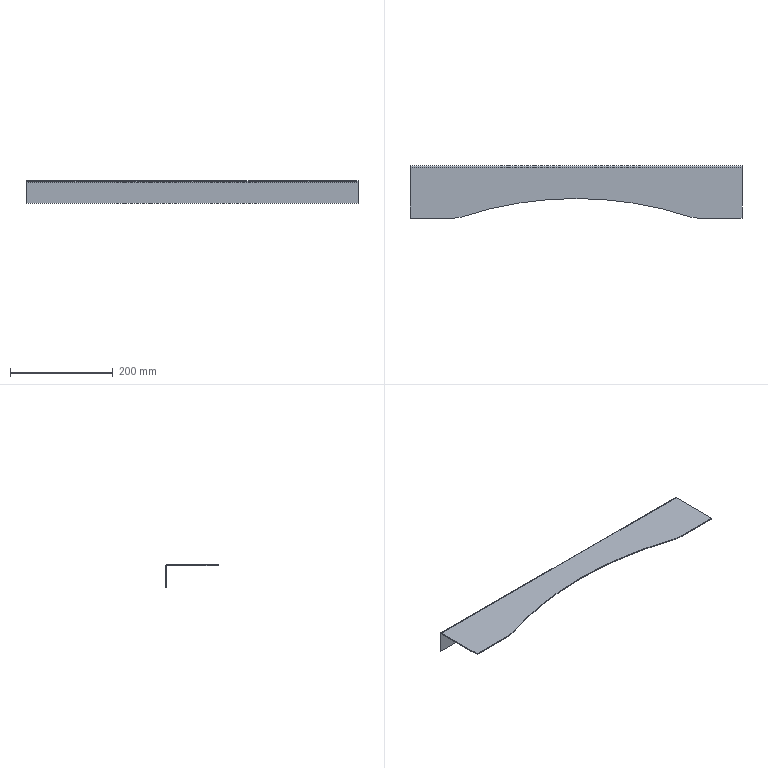Part | NX | features BREP 1 | 1 solid | 18 faces | box 646.176 x 101.6 x 44.45 mm | volume 151816 mm3 | plane 13 | cylinder 5 | commonest cylinder face diameters 127 x2 3.175 x1 6.934 x1 1410 x1
STEP:
#1=CARTESIAN_POINT('',(-238.949,0.,0.));
#2=VERTEX_POINT('',#1);
#3=CARTESIAN_POINT('',(-219.201,3.149,0.));
#4=VERTEX_POINT('',#3);
#5=CARTESIAN_POINT('',(-238.949,63.5,0.));
#6=DIRECTION('',(0.,0.,1.));
#7=DIRECTION('',(0.,-1.,0.));
#8=AXIS2_PLACEMENT_3D('',#5,#6,#7);
#9=CIRCLE('',#8,63.5);
#10=EDGE_CURVE('',#2,#4,#9,.T.);
#11=ORIENTED_EDGE('',*,*,#10,.T.);
#12=CARTESIAN_POINT('',(219.201,3.149,0.));
#13=VERTEX_POINT('',#12);
#14=CARTESIAN_POINT('',(0.,-666.75,0.));
#15=DIRECTION('',(0.,0.,1.));
#16=DIRECTION('',(0.311,0.9504,0.));
#17=AXIS2_PLACEMENT_3D('',#14,#15,#16);
#18=CIRCLE('',#17,704.85);
#19=EDGE_CURVE('',#13,#4,#18,.T.);
#20=ORIENTED_EDGE('',*,*,#19,.F.);
#21=CARTESIAN_POINT('',(238.949,0.,0.));
#22=VERTEX_POINT('',#21);
#23=CARTESIAN_POINT('',(238.949,63.5,0.));
#24=DIRECTION('',(0.,0.,1.));
#25=DIRECTION('',(-0.311,-0.9504,0.));
#26=AXIS2_PLACEMENT_3D('',#23,#24,#25);
#27=CIRCLE('',#26,63.5);
#28=EDGE_CURVE('',#13,#22,#27,.T.);
#29=ORIENTED_EDGE('',*,*,#28,.T.);
#30=CARTESIAN_POINT('',(323.088,0.,0.));
#31=VERTEX_POINT('',#30);
#32=CARTESIAN_POINT('',(238.949,0.,0.));
#33=DIRECTION('',(1.,0.,0.));
#34=VECTOR('',#33,1000.);
#35=LINE('',#32,#34);
#36=EDGE_CURVE('',#22,#31,#35,.T.);
#37=ORIENTED_EDGE('',*,*,#36,.T.);
#38=CARTESIAN_POINT('',(323.088,98.133,0.));
#39=VERTEX_POINT('',#38);
#40=CARTESIAN_POINT('',(323.088,0.,0.));
#41=DIRECTION('',(0.,1.,0.));
#42=VECTOR('',#41,1000.);
#43=LINE('',#40,#42);
#44=EDGE_CURVE('',#31,#39,#43,.T.);
#45=ORIENTED_EDGE('',*,*,#44,.T.);
#46=CARTESIAN_POINT('',(-323.088,98.133,0.));
#47=VERTEX_POINT('',#46);
#48=CARTESIAN_POINT('',(-323.088,98.133,0.));
#49=DIRECTION('',(1.,0.,0.));
#50=VECTOR('',#49,1000.);
#51=LINE('',#48,#50);
#52=EDGE_CURVE('',#47,#39,#51,.T.);
#53=ORIENTED_EDGE('',*,*,#52,.F.);
#54=CARTESIAN_POINT('',(-323.088,0.,0.));
#55=VERTEX_POINT('',#54);
#56=CARTESIAN_POINT('',(-323.088,98.133,0.));
#57=DIRECTION('',(0.,-1.,0.));
#58=VECTOR('',#57,1000.);
#59=LINE('',#56,#58);
#60=EDGE_CURVE('',#47,#55,#59,.T.);
#61=ORIENTED_EDGE('',*,*,#60,.T.);
#62=CARTESIAN_POINT('',(-323.088,0.,0.));
#63=DIRECTION('',(1.,0.,0.));
#64=VECTOR('',#63,1000.);
#65=LINE('',#62,#64);
#66=EDGE_CURVE('',#55,#2,#65,.T.);
#67=ORIENTED_EDGE('',*,*,#66,.T.);
#68=EDGE_LOOP('',(#11,#20,#29,#37,#45,#53,#61,#67));
#69=FACE_BOUND('',#68,.T.);
#70=CARTESIAN_POINT('',(0.,0.,0.));
#71=DIRECTION('',(0.,0.,1.));
#72=DIRECTION('',(1.,0.,0.));
#73=AXIS2_PLACEMENT_3D('',#70,#71,#72);
#74=PLANE('',#73);
#75=ADVANCED_FACE('',(#69),#74,.T.);
#76=CARTESIAN_POINT('',(-323.088,0.,-1.88));
#77=VERTEX_POINT('',#76);
#78=CARTESIAN_POINT('',(-323.088,0.,0.));
#79=DIRECTION('',(0.,0.,-1.));
#80=VECTOR('',#79,1000.);
#81=LINE('',#78,#80);
#82=EDGE_CURVE('',#55,#77,#81,.T.);
#83=ORIENTED_EDGE('',*,*,#82,.T.);
#84=CARTESIAN_POINT('',(-238.949,0.,-1.88));
#85=VERTEX_POINT('',#84);
#86=CARTESIAN_POINT('',(-323.088,0.,-1.88));
#87=DIRECTION('',(1.,0.,0.));
#88=VECTOR('',#87,1000.);
#89=LINE('',#86,#88);
#90=EDGE_CURVE('',#77,#85,#89,.T.);
#91=ORIENTED_EDGE('',*,*,#90,.T.);
#92=CARTESIAN_POINT('',(-238.949,0.,-1.88));
#93=DIRECTION('',(0.,0.,1.));
#94=VECTOR('',#93,1000.);
#95=LINE('',#92,#94);
#96=EDGE_CURVE('',#85,#2,#95,.T.);
#97=ORIENTED_EDGE('',*,*,#96,.T.);
#98=ORIENTED_EDGE('',*,*,#66,.F.);
#99=EDGE_LOOP('',(#83,#91,#97,#98));
#100=FACE_BOUND('',#99,.T.);
#101=CARTESIAN_POINT('',(0.,0.,-0.9398));
#102=DIRECTION('',(0.,-1.,0.));
#103=DIRECTION('',(0.,0.,-1.));
#104=AXIS2_PLACEMENT_3D('',#101,#102,#103);
#105=PLANE('',#104);
#106=ADVANCED_FACE('',(#100),#105,.T.);
#107=CARTESIAN_POINT('',(238.949,0.,-1.88));
#108=VERTEX_POINT('',#107);
#109=CARTESIAN_POINT('',(238.949,0.,-1.88));
#110=DIRECTION('',(0.,0.,1.));
#111=VECTOR('',#110,1000.);
#112=LINE('',#109,#111);
#113=EDGE_CURVE('',#108,#22,#112,.T.);
#114=ORIENTED_EDGE('',*,*,#113,.F.);
#115=CARTESIAN_POINT('',(323.088,0.,-1.88));
#116=VERTEX_POINT('',#115);
#117=CARTESIAN_POINT('',(238.949,0.,-1.88));
#118=DIRECTION('',(1.,0.,0.));
#119=VECTOR('',#118,1000.);
#120=LINE('',#117,#119);
#121=EDGE_CURVE('',#108,#116,#120,.T.);
#122=ORIENTED_EDGE('',*,*,#121,.T.);
#123=CARTESIAN_POINT('',(323.088,0.,0.));
#124=DIRECTION('',(0.,0.,-1.));
#125=VECTOR('',#124,1000.);
#126=LINE('',#123,#125);
#127=EDGE_CURVE('',#31,#116,#126,.T.);
#128=ORIENTED_EDGE('',*,*,#127,.F.);
#129=ORIENTED_EDGE('',*,*,#36,.F.);
#130=EDGE_LOOP('',(#114,#122,#128,#129));
#131=FACE_BOUND('',#130,.T.);
#132=CARTESIAN_POINT('',(0.,0.,-0.9398));
#133=DIRECTION('',(0.,-1.,0.));
#134=DIRECTION('',(0.,0.,-1.));
#135=AXIS2_PLACEMENT_3D('',#132,#133,#134);
#136=PLANE('',#135);
#137=ADVANCED_FACE('',(#131),#136,.T.);
#138=CARTESIAN_POINT('',(-219.201,3.149,-1.88));
#139=VERTEX_POINT('',#138);
#140=CARTESIAN_POINT('',(-238.949,63.5,-1.88));
#141=DIRECTION('',(0.,0.,-1.));
#142=DIRECTION('',(0.311,-0.9504,0.));
#143=AXIS2_PLACEMENT_3D('',#140,#141,#142);
#144=CIRCLE('',#143,63.5);
#145=EDGE_CURVE('',#139,#85,#144,.T.);
#146=ORIENTED_EDGE('',*,*,#145,.F.);
#147=CARTESIAN_POINT('',(-219.201,3.149,-1.88));
#148=DIRECTION('',(0.,0.,1.));
#149=VECTOR('',#148,1000.);
#150=LINE('',#147,#149);
#151=EDGE_CURVE('',#139,#4,#150,.T.);
#152=ORIENTED_EDGE('',*,*,#151,.T.);
#153=ORIENTED_EDGE('',*,*,#10,.F.);
#154=ORIENTED_EDGE('',*,*,#96,.F.);
#155=EDGE_LOOP('',(#146,#152,#153,#154));
#156=FACE_BOUND('',#155,.T.);
#157=CARTESIAN_POINT('',(-238.949,63.5,-2.756));
#158=DIRECTION('',(0.,0.,1.));
#159=DIRECTION('',(0.,-1.,0.));
#160=AXIS2_PLACEMENT_3D('',#157,#158,#159);
#161=CYLINDRICAL_SURFACE('',#160,63.5);
#162=ADVANCED_FACE('',(#156),#161,.T.);
#163=CARTESIAN_POINT('',(219.201,3.149,-1.88));
#164=VERTEX_POINT('',#163);
#165=CARTESIAN_POINT('',(0.,-666.75,-1.88));
#166=DIRECTION('',(0.,0.,1.));
#167=DIRECTION('',(0.311,0.9504,0.));
#168=AXIS2_PLACEMENT_3D('',#165,#166,#167);
#169=CIRCLE('',#168,704.85);
#170=EDGE_CURVE('',#164,#139,#169,.T.);
#171=ORIENTED_EDGE('',*,*,#170,.F.);
#172=CARTESIAN_POINT('',(219.201,3.149,-1.88));
#173=DIRECTION('',(0.,0.,1.));
#174=VECTOR('',#173,1000.);
#175=LINE('',#172,#174);
#176=EDGE_CURVE('',#164,#13,#175,.T.);
#177=ORIENTED_EDGE('',*,*,#176,.T.);
#178=ORIENTED_EDGE('',*,*,#19,.T.);
#179=ORIENTED_EDGE('',*,*,#151,.F.);
#180=EDGE_LOOP('',(#171,#177,#178,#179));
#181=FACE_BOUND('',#180,.T.);
#182=CARTESIAN_POINT('',(0.,-666.75,-0.9398));
#183=DIRECTION('',(0.,0.,1.));
#184=DIRECTION('',(0.3243,0.9459,0.));
#185=AXIS2_PLACEMENT_3D('',#182,#183,#184);
#186=CYLINDRICAL_SURFACE('',#185,704.85);
#187=ADVANCED_FACE('',(#181),#186,.F.);
#188=CARTESIAN_POINT('',(238.949,63.5,-1.88));
#189=DIRECTION('',(0.,0.,-1.));
#190=DIRECTION('',(0.,-1.,0.));
#191=AXIS2_PLACEMENT_3D('',#188,#189,#190);
#192=CIRCLE('',#191,63.5);
#193=EDGE_CURVE('',#108,#164,#192,.T.);
#194=ORIENTED_EDGE('',*,*,#193,.F.);
#195=ORIENTED_EDGE('',*,*,#113,.T.);
#196=ORIENTED_EDGE('',*,*,#28,.F.);
#197=ORIENTED_EDGE('',*,*,#176,.F.);
#198=EDGE_LOOP('',(#194,#195,#196,#197));
#199=FACE_BOUND('',#198,.T.);
#200=CARTESIAN_POINT('',(238.949,63.5,-2.756));
#201=DIRECTION('',(0.,0.,1.));
#202=DIRECTION('',(-0.311,-0.9504,0.));
#203=AXIS2_PLACEMENT_3D('',#200,#201,#202);
#204=CYLINDRICAL_SURFACE('',#203,63.5);
#205=ADVANCED_FACE('',(#199),#204,.T.);
#206=CARTESIAN_POINT('',(-323.088,98.133,-1.88));
#207=VERTEX_POINT('',#206);
#208=CARTESIAN_POINT('',(-323.088,98.133,-1.88));
#209=DIRECTION('',(0.,-1.,0.));
#210=VECTOR('',#209,1000.);
#211=LINE('',#208,#210);
#212=EDGE_CURVE('',#207,#77,#211,.T.);
#213=ORIENTED_EDGE('',*,*,#212,.F.);
#214=CARTESIAN_POINT('',(323.088,98.133,-1.88));
#215=VERTEX_POINT('',#214);
#216=CARTESIAN_POINT('',(-323.088,98.133,-1.88));
#217=DIRECTION('',(1.,0.,0.));
#218=VECTOR('',#217,1000.);
#219=LINE('',#216,#218);
#220=EDGE_CURVE('',#207,#215,#219,.T.);
#221=ORIENTED_EDGE('',*,*,#220,.T.);
#222=CARTESIAN_POINT('',(323.088,0.,-1.88));
#223=DIRECTION('',(0.,1.,0.));
#224=VECTOR('',#223,1000.);
#225=LINE('',#222,#224);
#226=EDGE_CURVE('',#116,#215,#225,.T.);
#227=ORIENTED_EDGE('',*,*,#226,.F.);
#228=ORIENTED_EDGE('',*,*,#121,.F.);
#229=ORIENTED_EDGE('',*,*,#193,.T.);
#230=ORIENTED_EDGE('',*,*,#170,.T.);
#231=ORIENTED_EDGE('',*,*,#145,.T.);
#232=ORIENTED_EDGE('',*,*,#90,.F.);
#233=EDGE_LOOP('',(#213,#221,#227,#228,#229,#230,#231,#232));
#234=FACE_BOUND('',#233,.T.);
#235=CARTESIAN_POINT('',(0.,0.,-1.88));
#236=DIRECTION('',(0.,0.,1.));
#237=DIRECTION('',(1.,0.,0.));
#238=AXIS2_PLACEMENT_3D('',#235,#236,#237);
#239=PLANE('',#238);
#240=ADVANCED_FACE('',(#234),#239,.F.);
#241=ORIENTED_EDGE('',*,*,#127,.T.);
#242=ORIENTED_EDGE('',*,*,#226,.T.);
#243=CARTESIAN_POINT('',(323.088,98.133,0.));
#244=DIRECTION('',(0.,0.,-1.));
#245=VECTOR('',#244,1000.);
#246=LINE('',#243,#245);
#247=EDGE_CURVE('',#39,#215,#246,.T.);
#248=ORIENTED_EDGE('',*,*,#247,.F.);
#249=ORIENTED_EDGE('',*,*,#44,.F.);
#250=EDGE_LOOP('',(#241,#242,#248,#249));
#251=FACE_BOUND('',#250,.T.);
#252=CARTESIAN_POINT('',(323.088,50.8,-0.9398));
#253=DIRECTION('',(1.,0.,0.));
#254=DIRECTION('',(0.,1.,0.));
#255=AXIS2_PLACEMENT_3D('',#252,#253,#254);
#256=PLANE('',#255);
#257=ADVANCED_FACE('',(#251),#256,.T.);
#258=ORIENTED_EDGE('',*,*,#247,.T.);
#259=CARTESIAN_POINT('',(323.088,99.72,-3.467));
#260=VERTEX_POINT('',#259);
#261=CARTESIAN_POINT('',(323.088,98.133,-3.467));
#262=DIRECTION('',(1.,0.,0.));
#263=DIRECTION('',(0.,1.,0.));
#264=AXIS2_PLACEMENT_3D('',#261,#262,#263);
#265=CIRCLE('',#264,1.588);
#266=EDGE_CURVE('',#260,#215,#265,.T.);
#267=ORIENTED_EDGE('',*,*,#266,.F.);
#268=CARTESIAN_POINT('',(323.088,101.6,-3.467));
#269=VERTEX_POINT('',#268);
#270=CARTESIAN_POINT('',(323.088,101.6,-3.467));
#271=DIRECTION('',(0.,-1.,0.));
#272=VECTOR('',#271,1000.);
#273=LINE('',#270,#272);
#274=EDGE_CURVE('',#269,#260,#273,.T.);
#275=ORIENTED_EDGE('',*,*,#274,.F.);
#276=CARTESIAN_POINT('',(323.088,98.133,-3.467));
#277=DIRECTION('',(1.,0.,0.));
#278=DIRECTION('',(0.,1.,0.));
#279=AXIS2_PLACEMENT_3D('',#276,#277,#278);
#280=CIRCLE('',#279,3.467);
#281=EDGE_CURVE('',#269,#39,#280,.T.);
#282=ORIENTED_EDGE('',*,*,#281,.T.);
#283=EDGE_LOOP('',(#258,#267,#275,#282));
#284=FACE_BOUND('',#283,.T.);
#285=CARTESIAN_POINT('',(323.088,99.92,-1.68));
#286=DIRECTION('',(-1.,0.,0.));
#287=DIRECTION('',(0.,0.,1.));
#288=AXIS2_PLACEMENT_3D('',#285,#286,#287);
#289=PLANE('',#288);
#290=ADVANCED_FACE('',(#284),#289,.F.);
#291=CARTESIAN_POINT('',(-323.088,101.6,-3.467));
#292=VERTEX_POINT('',#291);
#293=CARTESIAN_POINT('',(-323.088,98.133,-3.467));
#294=DIRECTION('',(1.,0.,0.));
#295=DIRECTION('',(0.,1.,0.));
#296=AXIS2_PLACEMENT_3D('',#293,#294,#295);
#297=CIRCLE('',#296,3.467);
#298=EDGE_CURVE('',#292,#47,#297,.T.);
#299=ORIENTED_EDGE('',*,*,#298,.T.);
#300=ORIENTED_EDGE('',*,*,#52,.T.);
#301=ORIENTED_EDGE('',*,*,#281,.F.);
#302=CARTESIAN_POINT('',(-323.088,101.6,-3.467));
#303=DIRECTION('',(1.,0.,0.));
#304=VECTOR('',#303,1000.);
#305=LINE('',#302,#304);
#306=EDGE_CURVE('',#292,#269,#305,.T.);
#307=ORIENTED_EDGE('',*,*,#306,.F.);
#308=EDGE_LOOP('',(#299,#300,#301,#307));
#309=FACE_BOUND('',#308,.T.);
#310=CARTESIAN_POINT('',(-323.088,98.133,-3.467));
#311=DIRECTION('',(1.,0.,0.));
#312=DIRECTION('',(0.,1.,0.));
#313=AXIS2_PLACEMENT_3D('',#310,#311,#312);
#314=CYLINDRICAL_SURFACE('',#313,3.467);
#315=ADVANCED_FACE('',(#309),#314,.T.);
#316=CARTESIAN_POINT('',(323.088,101.6,-44.45));
#317=VERTEX_POINT('',#316);
#318=CARTESIAN_POINT('',(-323.088,101.6,-44.45));
#319=VERTEX_POINT('',#318);
#320=CARTESIAN_POINT('',(323.088,101.6,-44.45));
#321=DIRECTION('',(-1.,0.,0.));
#322=VECTOR('',#321,1000.);
#323=LINE('',#320,#322);
#324=EDGE_CURVE('',#317,#319,#323,.T.);
#325=ORIENTED_EDGE('',*,*,#324,.T.);
#326=CARTESIAN_POINT('',(-323.088,101.6,-44.45));
#327=DIRECTION('',(0.,0.,1.));
#328=VECTOR('',#327,1000.);
#329=LINE('',#326,#328);
#330=EDGE_CURVE('',#319,#292,#329,.T.);
#331=ORIENTED_EDGE('',*,*,#330,.T.);
#332=ORIENTED_EDGE('',*,*,#306,.T.);
#333=CARTESIAN_POINT('',(323.088,101.6,-3.467));
#334=DIRECTION('',(0.,0.,-1.));
#335=VECTOR('',#334,1000.);
#336=LINE('',#333,#335);
#337=EDGE_CURVE('',#269,#317,#336,.T.);
#338=ORIENTED_EDGE('',*,*,#337,.T.);
#339=EDGE_LOOP('',(#325,#331,#332,#338));
#340=FACE_BOUND('',#339,.T.);
#341=CARTESIAN_POINT('',(169.557,101.6,0.));
#342=DIRECTION('',(0.,1.,0.));
#343=DIRECTION('',(1.,0.,0.));
#344=AXIS2_PLACEMENT_3D('',#341,#342,#343);
#345=PLANE('',#344);
#346=ADVANCED_FACE('',(#340),#345,.T.);
#347=ORIENTED_EDGE('',*,*,#274,.T.);
#348=CARTESIAN_POINT('',(323.088,99.72,-44.45));
#349=VERTEX_POINT('',#348);
#350=CARTESIAN_POINT('',(323.088,99.72,-3.467));
#351=DIRECTION('',(0.,0.,-1.));
#352=VECTOR('',#351,1000.);
#353=LINE('',#350,#352);
#354=EDGE_CURVE('',#260,#349,#353,.T.);
#355=ORIENTED_EDGE('',*,*,#354,.T.);
#356=CARTESIAN_POINT('',(323.088,101.6,-44.45));
#357=DIRECTION('',(0.,-1.,0.));
#358=VECTOR('',#357,1000.);
#359=LINE('',#356,#358);
#360=EDGE_CURVE('',#317,#349,#359,.T.);
#361=ORIENTED_EDGE('',*,*,#360,.F.);
#362=ORIENTED_EDGE('',*,*,#337,.F.);
#363=EDGE_LOOP('',(#347,#355,#361,#362));
#364=FACE_BOUND('',#363,.T.);
#365=CARTESIAN_POINT('',(323.088,100.66,-23.959));
#366=DIRECTION('',(1.,0.,0.));
#367=DIRECTION('',(0.,1.,0.));
#368=AXIS2_PLACEMENT_3D('',#365,#366,#367);
#369=PLANE('',#368);
#370=ADVANCED_FACE('',(#364),#369,.T.);
#371=ORIENTED_EDGE('',*,*,#360,.T.);
#372=CARTESIAN_POINT('',(-323.088,99.72,-44.45));
#373=VERTEX_POINT('',#372);
#374=CARTESIAN_POINT('',(323.088,99.72,-44.45));
#375=DIRECTION('',(-1.,0.,0.));
#376=VECTOR('',#375,1000.);
#377=LINE('',#374,#376);
#378=EDGE_CURVE('',#349,#373,#377,.T.);
#379=ORIENTED_EDGE('',*,*,#378,.T.);
#380=CARTESIAN_POINT('',(-323.088,101.6,-44.45));
#381=DIRECTION('',(0.,-1.,0.));
#382=VECTOR('',#381,1000.);
#383=LINE('',#380,#382);
#384=EDGE_CURVE('',#319,#373,#383,.T.);
#385=ORIENTED_EDGE('',*,*,#384,.F.);
#386=ORIENTED_EDGE('',*,*,#324,.F.);
#387=EDGE_LOOP('',(#371,#379,#385,#386));
#388=FACE_BOUND('',#387,.T.);
#389=CARTESIAN_POINT('',(0.,100.66,-44.45));
#390=DIRECTION('',(0.,0.,-1.));
#391=DIRECTION('',(0.,-1.,0.));
#392=AXIS2_PLACEMENT_3D('',#389,#390,#391);
#393=PLANE('',#392);
#394=ADVANCED_FACE('',(#388),#393,.T.);
#395=ORIENTED_EDGE('',*,*,#384,.T.);
#396=CARTESIAN_POINT('',(-323.088,99.72,-3.467));
#397=VERTEX_POINT('',#396);
#398=CARTESIAN_POINT('',(-323.088,99.72,-44.45));
#399=DIRECTION('',(0.,0.,1.));
#400=VECTOR('',#399,1000.);
#401=LINE('',#398,#400);
#402=EDGE_CURVE('',#373,#397,#401,.T.);
#403=ORIENTED_EDGE('',*,*,#402,.T.);
#404=CARTESIAN_POINT('',(-323.088,101.6,-3.467));
#405=DIRECTION('',(0.,-1.,0.));
#406=VECTOR('',#405,1000.);
#407=LINE('',#404,#406);
#408=EDGE_CURVE('',#292,#397,#407,.T.);
#409=ORIENTED_EDGE('',*,*,#408,.F.);
#410=ORIENTED_EDGE('',*,*,#330,.F.);
#411=EDGE_LOOP('',(#395,#403,#409,#410));
#412=FACE_BOUND('',#411,.T.);
#413=CARTESIAN_POINT('',(-323.088,100.66,-23.959));
#414=DIRECTION('',(-1.,0.,0.));
#415=DIRECTION('',(0.,0.,1.));
#416=AXIS2_PLACEMENT_3D('',#413,#414,#415);
#417=PLANE('',#416);
#418=ADVANCED_FACE('',(#412),#417,.T.);
#419=ORIENTED_EDGE('',*,*,#408,.T.);
#420=CARTESIAN_POINT('',(-323.088,98.133,-3.467));
#421=DIRECTION('',(1.,0.,0.));
#422=DIRECTION('',(0.,1.,0.));
#423=AXIS2_PLACEMENT_3D('',#420,#421,#422);
#424=CIRCLE('',#423,1.588);
#425=EDGE_CURVE('',#397,#207,#424,.T.);
#426=ORIENTED_EDGE('',*,*,#425,.T.);
#427=CARTESIAN_POINT('',(-323.088,98.133,0.));
#428=DIRECTION('',(0.,0.,-1.));
#429=VECTOR('',#428,1000.);
#430=LINE('',#427,#429);
#431=EDGE_CURVE('',#47,#207,#430,.T.);
#432=ORIENTED_EDGE('',*,*,#431,.F.);
#433=ORIENTED_EDGE('',*,*,#298,.F.);
#434=EDGE_LOOP('',(#419,#426,#432,#433));
#435=FACE_BOUND('',#434,.T.);
#436=CARTESIAN_POINT('',(-323.088,99.92,-1.68));
#437=DIRECTION('',(-1.,0.,0.));
#438=DIRECTION('',(0.,0.,1.));
#439=AXIS2_PLACEMENT_3D('',#436,#437,#438);
#440=PLANE('',#439);
#441=ADVANCED_FACE('',(#435),#440,.T.);
#442=ORIENTED_EDGE('',*,*,#431,.T.);
#443=ORIENTED_EDGE('',*,*,#212,.T.);
#444=ORIENTED_EDGE('',*,*,#82,.F.);
#445=ORIENTED_EDGE('',*,*,#60,.F.);
#446=EDGE_LOOP('',(#442,#443,#444,#445));
#447=FACE_BOUND('',#446,.T.);
#448=CARTESIAN_POINT('',(-323.088,50.8,-0.9398));
#449=DIRECTION('',(-1.,0.,0.));
#450=DIRECTION('',(0.,0.,1.));
#451=AXIS2_PLACEMENT_3D('',#448,#449,#450);
#452=PLANE('',#451);
#453=ADVANCED_FACE('',(#447),#452,.T.);
#454=ORIENTED_EDGE('',*,*,#266,.T.);
#455=ORIENTED_EDGE('',*,*,#220,.F.);
#456=ORIENTED_EDGE('',*,*,#425,.F.);
#457=CARTESIAN_POINT('',(-323.088,99.72,-3.467));
#458=DIRECTION('',(1.,0.,0.));
#459=VECTOR('',#458,1000.);
#460=LINE('',#457,#459);
#461=EDGE_CURVE('',#397,#260,#460,.T.);
#462=ORIENTED_EDGE('',*,*,#461,.T.);
#463=EDGE_LOOP('',(#454,#455,#456,#462));
#464=FACE_BOUND('',#463,.T.);
#465=CARTESIAN_POINT('',(-323.088,98.133,-3.467));
#466=DIRECTION('',(1.,0.,0.));
#467=DIRECTION('',(0.,1.,0.));
#468=AXIS2_PLACEMENT_3D('',#465,#466,#467);
#469=CYLINDRICAL_SURFACE('',#468,1.588);
#470=ADVANCED_FACE('',(#464),#469,.F.);
#471=ORIENTED_EDGE('',*,*,#461,.F.);
#472=ORIENTED_EDGE('',*,*,#402,.F.);
#473=ORIENTED_EDGE('',*,*,#378,.F.);
#474=ORIENTED_EDGE('',*,*,#354,.F.);
#475=EDGE_LOOP('',(#471,#472,#473,#474));
#476=FACE_BOUND('',#475,.T.);
#477=CARTESIAN_POINT('',(169.557,99.72,0.));
#478=DIRECTION('',(0.,1.,0.));
#479=DIRECTION('',(1.,0.,0.));
#480=AXIS2_PLACEMENT_3D('',#477,#478,#479);
#481=PLANE('',#480);
#482=ADVANCED_FACE('',(#476),#481,.F.);
#483=CLOSED_SHELL('',(#75,#106,#137,#162,#187,#205,#240,#257,#290,#315,#346,#370,#394,#418,#441,#453,#470,#482));
#484=MANIFOLD_SOLID_BREP('',#483);
#485=(LENGTH_UNIT()NAMED_UNIT(*)SI_UNIT(.MILLI.,.METRE.));
#486=UNCERTAINTY_MEASURE_WITH_UNIT(LENGTH_MEASURE(0.00001),#485,'','');
#487=(NAMED_UNIT(*)PLANE_ANGLE_UNIT()SI_UNIT($,.RADIAN.));
#488=(NAMED_UNIT(*)SI_UNIT($,.STERADIAN.)SOLID_ANGLE_UNIT());
#489=(GEOMETRIC_REPRESENTATION_CONTEXT(3)GLOBAL_UNCERTAINTY_ASSIGNED_CONTEXT((#486))GLOBAL_UNIT_ASSIGNED_CONTEXT((#485,#487,#488))REPRESENTATION_CONTEXT('',''));
#490=ADVANCED_BREP_SHAPE_REPRESENTATION('',(#484),#489);